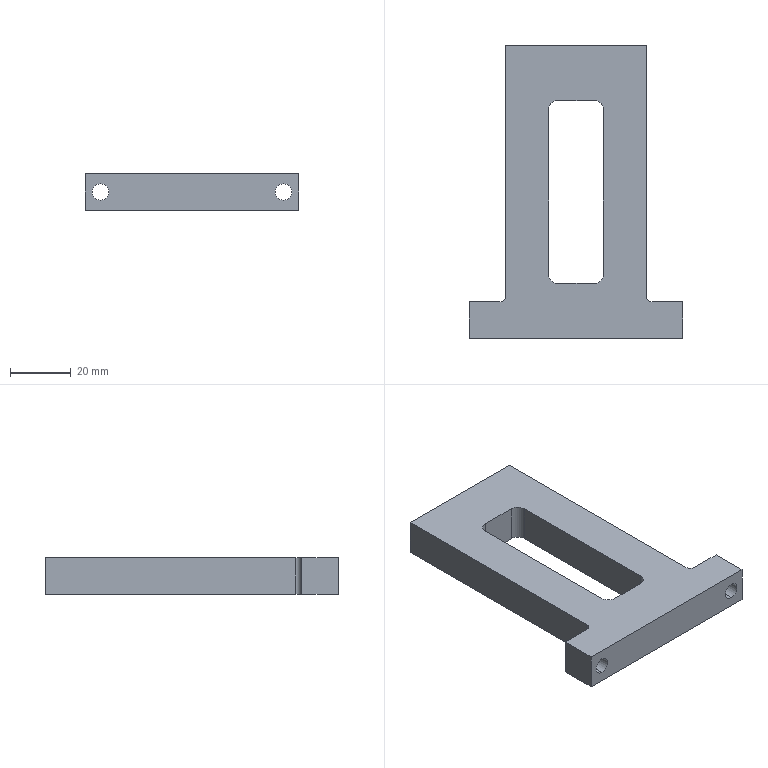Part | STEP file | 11-FG-E02011 | 1 solid | 36 faces | box 70 x 96 x 12 mm | volume 42748 mm3 | cylinder 16 | plane 14 | cone 6 | commonest cylinder face diameters 3.3 x6 5.4 x4 6 x4 4 x2
STEP:
#1=CARTESIAN_POINT('',(-17.,36.5,-1.65));
#2=VERTEX_POINT('',#1);
#3=CARTESIAN_POINT('',(-17.,36.5,1.65));
#4=VERTEX_POINT('',#3);
#5=CARTESIAN_POINT('',(-17.,36.5,0.));
#6=DIRECTION('',(0.,1.,0.));
#7=DIRECTION('',(0.,0.,1.));
#8=AXIS2_PLACEMENT_3D('',#5,#6,#7);
#9=CIRCLE('',#8,1.65);
#10=EDGE_CURVE('',#2,#4,#9,.T.);
#11=ORIENTED_EDGE('',*,*,#10,.F.);
#12=CARTESIAN_POINT('',(-17.,48.,-1.65));
#13=VERTEX_POINT('',#12);
#14=CARTESIAN_POINT('',(-17.,48.,-1.65));
#15=DIRECTION('',(0.,1.,0.));
#16=VECTOR('',#15,1000.);
#17=LINE('',#14,#16);
#18=EDGE_CURVE('',#2,#13,#17,.T.);
#19=ORIENTED_EDGE('',*,*,#18,.T.);
#20=CARTESIAN_POINT('',(-17.,48.,1.65));
#21=VERTEX_POINT('',#20);
#22=CARTESIAN_POINT('',(-17.,48.,0.));
#23=DIRECTION('',(0.,1.,0.));
#24=DIRECTION('',(0.,0.,1.));
#25=AXIS2_PLACEMENT_3D('',#22,#23,#24);
#26=CIRCLE('',#25,1.65);
#27=EDGE_CURVE('',#13,#21,#26,.T.);
#28=ORIENTED_EDGE('',*,*,#27,.T.);
#29=CARTESIAN_POINT('',(-17.,48.,1.65));
#30=DIRECTION('',(0.,1.,0.));
#31=VECTOR('',#30,1000.);
#32=LINE('',#29,#31);
#33=EDGE_CURVE('',#4,#21,#32,.T.);
#34=ORIENTED_EDGE('',*,*,#33,.F.);
#35=EDGE_LOOP('',(#11,#19,#28,#34));
#36=FACE_OUTER_BOUND('',#35,.T.);
#37=CARTESIAN_POINT('',(-17.,48.,0.));
#38=DIRECTION('',(0.,1.,0.));
#39=DIRECTION('',(0.,0.,1.));
#40=AXIS2_PLACEMENT_3D('',#37,#38,#39);
#41=CYLINDRICAL_SURFACE('',#40,1.65);
#42=ADVANCED_FACE('',(#36),#41,.F.);
#43=CARTESIAN_POINT('',(-17.,35.509,0.));
#44=VERTEX_POINT('',#43);
#45=CARTESIAN_POINT('',(-17.,36.5,1.65));
#46=DIRECTION('',(0.,0.515,0.8572));
#47=VECTOR('',#46,1000.);
#48=LINE('',#45,#47);
#49=EDGE_CURVE('',#44,#4,#48,.T.);
#50=ORIENTED_EDGE('',*,*,#49,.F.);
#51=CARTESIAN_POINT('',(-17.,36.5,-1.65));
#52=DIRECTION('',(0.,0.515,-0.8572));
#53=VECTOR('',#52,1000.);
#54=LINE('',#51,#53);
#55=EDGE_CURVE('',#44,#2,#54,.T.);
#56=ORIENTED_EDGE('',*,*,#55,.T.);
#57=ORIENTED_EDGE('',*,*,#10,.T.);
#58=EDGE_LOOP('',(#50,#56,#57));
#59=FACE_OUTER_BOUND('',#58,.T.);
#60=CARTESIAN_POINT('',(-17.,36.5,0.));
#61=DIRECTION('',(0.,1.,0.));
#62=DIRECTION('',(0.,0.,1.));
#63=AXIS2_PLACEMENT_3D('',#60,#61,#62);
#64=CONICAL_SURFACE('',#63,1.65,1.03);
#65=ADVANCED_FACE('',(#59),#64,.F.);
#66=CARTESIAN_POINT('',(0.,36.5,-1.65));
#67=VERTEX_POINT('',#66);
#68=CARTESIAN_POINT('',(0.,36.5,1.65));
#69=VERTEX_POINT('',#68);
#70=CARTESIAN_POINT('',(0.,36.5,0.));
#71=DIRECTION('',(0.,1.,0.));
#72=DIRECTION('',(0.,0.,1.));
#73=AXIS2_PLACEMENT_3D('',#70,#71,#72);
#74=CIRCLE('',#73,1.65);
#75=EDGE_CURVE('',#67,#69,#74,.T.);
#76=ORIENTED_EDGE('',*,*,#75,.F.);
#77=CARTESIAN_POINT('',(0.,48.,-1.65));
#78=VERTEX_POINT('',#77);
#79=CARTESIAN_POINT('',(0.,48.,-1.65));
#80=DIRECTION('',(0.,1.,0.));
#81=VECTOR('',#80,1000.);
#82=LINE('',#79,#81);
#83=EDGE_CURVE('',#67,#78,#82,.T.);
#84=ORIENTED_EDGE('',*,*,#83,.T.);
#85=CARTESIAN_POINT('',(0.,48.,1.65));
#86=VERTEX_POINT('',#85);
#87=CARTESIAN_POINT('',(0.,48.,0.));
#88=DIRECTION('',(0.,1.,0.));
#89=DIRECTION('',(0.,0.,1.));
#90=AXIS2_PLACEMENT_3D('',#87,#88,#89);
#91=CIRCLE('',#90,1.65);
#92=EDGE_CURVE('',#78,#86,#91,.T.);
#93=ORIENTED_EDGE('',*,*,#92,.T.);
#94=CARTESIAN_POINT('',(0.,48.,1.65));
#95=DIRECTION('',(0.,1.,0.));
#96=VECTOR('',#95,1000.);
#97=LINE('',#94,#96);
#98=EDGE_CURVE('',#69,#86,#97,.T.);
#99=ORIENTED_EDGE('',*,*,#98,.F.);
#100=EDGE_LOOP('',(#76,#84,#93,#99));
#101=FACE_OUTER_BOUND('',#100,.T.);
#102=CARTESIAN_POINT('',(0.,48.,0.));
#103=DIRECTION('',(0.,1.,0.));
#104=DIRECTION('',(0.,0.,1.));
#105=AXIS2_PLACEMENT_3D('',#102,#103,#104);
#106=CYLINDRICAL_SURFACE('',#105,1.65);
#107=ADVANCED_FACE('',(#101),#106,.F.);
#108=CARTESIAN_POINT('',(0.,35.509,0.));
#109=VERTEX_POINT('',#108);
#110=CARTESIAN_POINT('',(0.,36.5,1.65));
#111=DIRECTION('',(0.,0.515,0.8572));
#112=VECTOR('',#111,1000.);
#113=LINE('',#110,#112);
#114=EDGE_CURVE('',#109,#69,#113,.T.);
#115=ORIENTED_EDGE('',*,*,#114,.F.);
#116=CARTESIAN_POINT('',(0.,36.5,-1.65));
#117=DIRECTION('',(0.,0.515,-0.8572));
#118=VECTOR('',#117,1000.);
#119=LINE('',#116,#118);
#120=EDGE_CURVE('',#109,#67,#119,.T.);
#121=ORIENTED_EDGE('',*,*,#120,.T.);
#122=ORIENTED_EDGE('',*,*,#75,.T.);
#123=EDGE_LOOP('',(#115,#121,#122));
#124=FACE_OUTER_BOUND('',#123,.T.);
#125=CARTESIAN_POINT('',(0.,36.5,0.));
#126=DIRECTION('',(0.,1.,0.));
#127=DIRECTION('',(0.,0.,1.));
#128=AXIS2_PLACEMENT_3D('',#125,#126,#127);
#129=CONICAL_SURFACE('',#128,1.65,1.03);
#130=ADVANCED_FACE('',(#124),#129,.F.);
#131=CARTESIAN_POINT('',(17.,36.5,-1.65));
#132=VERTEX_POINT('',#131);
#133=CARTESIAN_POINT('',(17.,36.5,1.65));
#134=VERTEX_POINT('',#133);
#135=CARTESIAN_POINT('',(17.,36.5,0.));
#136=DIRECTION('',(0.,1.,0.));
#137=DIRECTION('',(0.,0.,1.));
#138=AXIS2_PLACEMENT_3D('',#135,#136,#137);
#139=CIRCLE('',#138,1.65);
#140=EDGE_CURVE('',#132,#134,#139,.T.);
#141=ORIENTED_EDGE('',*,*,#140,.F.);
#142=CARTESIAN_POINT('',(17.,48.,-1.65));
#143=VERTEX_POINT('',#142);
#144=CARTESIAN_POINT('',(17.,48.,-1.65));
#145=DIRECTION('',(0.,1.,0.));
#146=VECTOR('',#145,1000.);
#147=LINE('',#144,#146);
#148=EDGE_CURVE('',#132,#143,#147,.T.);
#149=ORIENTED_EDGE('',*,*,#148,.T.);
#150=CARTESIAN_POINT('',(17.,48.,1.65));
#151=VERTEX_POINT('',#150);
#152=CARTESIAN_POINT('',(17.,48.,0.));
#153=DIRECTION('',(0.,1.,0.));
#154=DIRECTION('',(0.,0.,1.));
#155=AXIS2_PLACEMENT_3D('',#152,#153,#154);
#156=CIRCLE('',#155,1.65);
#157=EDGE_CURVE('',#143,#151,#156,.T.);
#158=ORIENTED_EDGE('',*,*,#157,.T.);
#159=CARTESIAN_POINT('',(17.,48.,1.65));
#160=DIRECTION('',(0.,1.,0.));
#161=VECTOR('',#160,1000.);
#162=LINE('',#159,#161);
#163=EDGE_CURVE('',#134,#151,#162,.T.);
#164=ORIENTED_EDGE('',*,*,#163,.F.);
#165=EDGE_LOOP('',(#141,#149,#158,#164));
#166=FACE_OUTER_BOUND('',#165,.T.);
#167=CARTESIAN_POINT('',(17.,48.,0.));
#168=DIRECTION('',(0.,1.,0.));
#169=DIRECTION('',(0.,0.,1.));
#170=AXIS2_PLACEMENT_3D('',#167,#168,#169);
#171=CYLINDRICAL_SURFACE('',#170,1.65);
#172=ADVANCED_FACE('',(#166),#171,.F.);
#173=CARTESIAN_POINT('',(17.,35.509,0.));
#174=VERTEX_POINT('',#173);
#175=CARTESIAN_POINT('',(17.,36.5,1.65));
#176=DIRECTION('',(0.,0.515,0.8572));
#177=VECTOR('',#176,1000.);
#178=LINE('',#175,#177);
#179=EDGE_CURVE('',#174,#134,#178,.T.);
#180=ORIENTED_EDGE('',*,*,#179,.F.);
#181=CARTESIAN_POINT('',(17.,36.5,-1.65));
#182=DIRECTION('',(0.,0.515,-0.8572));
#183=VECTOR('',#182,1000.);
#184=LINE('',#181,#183);
#185=EDGE_CURVE('',#174,#132,#184,.T.);
#186=ORIENTED_EDGE('',*,*,#185,.T.);
#187=ORIENTED_EDGE('',*,*,#140,.T.);
#188=EDGE_LOOP('',(#180,#186,#187));
#189=FACE_OUTER_BOUND('',#188,.T.);
#190=CARTESIAN_POINT('',(17.,36.5,0.));
#191=DIRECTION('',(0.,1.,0.));
#192=DIRECTION('',(0.,0.,1.));
#193=AXIS2_PLACEMENT_3D('',#190,#191,#192);
#194=CONICAL_SURFACE('',#193,1.65,1.03);
#195=ADVANCED_FACE('',(#189),#194,.F.);
#196=CARTESIAN_POINT('',(30.,-48.,-2.7));
#197=VERTEX_POINT('',#196);
#198=CARTESIAN_POINT('',(30.,-48.,2.7));
#199=VERTEX_POINT('',#198);
#200=CARTESIAN_POINT('',(30.,-48.,0.));
#201=DIRECTION('',(0.,1.,0.));
#202=DIRECTION('',(0.,0.,1.));
#203=AXIS2_PLACEMENT_3D('',#200,#201,#202);
#204=CIRCLE('',#203,2.7);
#205=EDGE_CURVE('',#197,#199,#204,.T.);
#206=ORIENTED_EDGE('',*,*,#205,.F.);
#207=CARTESIAN_POINT('',(30.,-36.,-2.7));
#208=VERTEX_POINT('',#207);
#209=CARTESIAN_POINT('',(30.,-36.,-2.7));
#210=DIRECTION('',(0.,1.,0.));
#211=VECTOR('',#210,1000.);
#212=LINE('',#209,#211);
#213=EDGE_CURVE('',#197,#208,#212,.T.);
#214=ORIENTED_EDGE('',*,*,#213,.T.);
#215=CARTESIAN_POINT('',(30.,-36.,2.7));
#216=VERTEX_POINT('',#215);
#217=CARTESIAN_POINT('',(30.,-36.,0.));
#218=DIRECTION('',(0.,1.,0.));
#219=DIRECTION('',(0.,0.,1.));
#220=AXIS2_PLACEMENT_3D('',#217,#218,#219);
#221=CIRCLE('',#220,2.7);
#222=EDGE_CURVE('',#208,#216,#221,.T.);
#223=ORIENTED_EDGE('',*,*,#222,.T.);
#224=CARTESIAN_POINT('',(30.,-36.,2.7));
#225=DIRECTION('',(0.,1.,0.));
#226=VECTOR('',#225,1000.);
#227=LINE('',#224,#226);
#228=EDGE_CURVE('',#199,#216,#227,.T.);
#229=ORIENTED_EDGE('',*,*,#228,.F.);
#230=EDGE_LOOP('',(#206,#214,#223,#229));
#231=FACE_OUTER_BOUND('',#230,.T.);
#232=CARTESIAN_POINT('',(30.,-36.,0.));
#233=DIRECTION('',(0.,1.,0.));
#234=DIRECTION('',(0.,0.,1.));
#235=AXIS2_PLACEMENT_3D('',#232,#233,#234);
#236=CYLINDRICAL_SURFACE('',#235,2.7);
#237=ADVANCED_FACE('',(#231),#236,.F.);
#238=CARTESIAN_POINT('',(-30.,-48.,-2.7));
#239=VERTEX_POINT('',#238);
#240=CARTESIAN_POINT('',(-30.,-48.,2.7));
#241=VERTEX_POINT('',#240);
#242=CARTESIAN_POINT('',(-30.,-48.,0.));
#243=DIRECTION('',(0.,1.,0.));
#244=DIRECTION('',(0.,0.,1.));
#245=AXIS2_PLACEMENT_3D('',#242,#243,#244);
#246=CIRCLE('',#245,2.7);
#247=EDGE_CURVE('',#239,#241,#246,.T.);
#248=ORIENTED_EDGE('',*,*,#247,.F.);
#249=CARTESIAN_POINT('',(-30.,-36.,-2.7));
#250=VERTEX_POINT('',#249);
#251=CARTESIAN_POINT('',(-30.,-36.,-2.7));
#252=DIRECTION('',(0.,1.,0.));
#253=VECTOR('',#252,1000.);
#254=LINE('',#251,#253);
#255=EDGE_CURVE('',#239,#250,#254,.T.);
#256=ORIENTED_EDGE('',*,*,#255,.T.);
#257=CARTESIAN_POINT('',(-30.,-36.,2.7));
#258=VERTEX_POINT('',#257);
#259=CARTESIAN_POINT('',(-30.,-36.,0.));
#260=DIRECTION('',(0.,1.,0.));
#261=DIRECTION('',(0.,0.,1.));
#262=AXIS2_PLACEMENT_3D('',#259,#260,#261);
#263=CIRCLE('',#262,2.7);
#264=EDGE_CURVE('',#250,#258,#263,.T.);
#265=ORIENTED_EDGE('',*,*,#264,.T.);
#266=CARTESIAN_POINT('',(-30.,-36.,2.7));
#267=DIRECTION('',(0.,1.,0.));
#268=VECTOR('',#267,1000.);
#269=LINE('',#266,#268);
#270=EDGE_CURVE('',#241,#258,#269,.T.);
#271=ORIENTED_EDGE('',*,*,#270,.F.);
#272=EDGE_LOOP('',(#248,#256,#265,#271));
#273=FACE_OUTER_BOUND('',#272,.T.);
#274=CARTESIAN_POINT('',(-30.,-36.,0.));
#275=DIRECTION('',(0.,1.,0.));
#276=DIRECTION('',(0.,0.,1.));
#277=AXIS2_PLACEMENT_3D('',#274,#275,#276);
#278=CYLINDRICAL_SURFACE('',#277,2.7);
#279=ADVANCED_FACE('',(#273),#278,.F.);
#280=CARTESIAN_POINT('',(35.,-48.,-6.));
#281=VERTEX_POINT('',#280);
#282=CARTESIAN_POINT('',(35.,-36.,-6.));
#283=VERTEX_POINT('',#282);
#284=CARTESIAN_POINT('',(35.,-48.,-6.));
#285=DIRECTION('',(0.,1.,0.));
#286=VECTOR('',#285,1000.);
#287=LINE('',#284,#286);
#288=EDGE_CURVE('',#281,#283,#287,.T.);
#289=ORIENTED_EDGE('',*,*,#288,.T.);
#290=CARTESIAN_POINT('',(35.,-36.,6.));
#291=VERTEX_POINT('',#290);
#292=CARTESIAN_POINT('',(35.,-36.,-6.));
#293=DIRECTION('',(0.,0.,1.));
#294=VECTOR('',#293,1000.);
#295=LINE('',#292,#294);
#296=EDGE_CURVE('',#283,#291,#295,.T.);
#297=ORIENTED_EDGE('',*,*,#296,.T.);
#298=CARTESIAN_POINT('',(35.,-48.,6.));
#299=VERTEX_POINT('',#298);
#300=CARTESIAN_POINT('',(35.,-48.,6.));
#301=DIRECTION('',(0.,1.,0.));
#302=VECTOR('',#301,1000.);
#303=LINE('',#300,#302);
#304=EDGE_CURVE('',#299,#291,#303,.T.);
#305=ORIENTED_EDGE('',*,*,#304,.F.);
#306=CARTESIAN_POINT('',(35.,-48.,6.));
#307=DIRECTION('',(0.,0.,-1.));
#308=VECTOR('',#307,1000.);
#309=LINE('',#306,#308);
#310=EDGE_CURVE('',#299,#281,#309,.T.);
#311=ORIENTED_EDGE('',*,*,#310,.T.);
#312=EDGE_LOOP('',(#289,#297,#305,#311));
#313=FACE_OUTER_BOUND('',#312,.T.);
#314=CARTESIAN_POINT('',(35.,-48.,6.));
#315=DIRECTION('',(-1.,0.,0.));
#316=DIRECTION('',(0.,0.,1.));
#317=AXIS2_PLACEMENT_3D('',#314,#315,#316);
#318=PLANE('',#317);
#319=ADVANCED_FACE('',(#313),#318,.F.);
#320=CARTESIAN_POINT('',(-17.,48.,0.));
#321=DIRECTION('',(0.,1.,0.));
#322=DIRECTION('',(0.,0.,1.));
#323=AXIS2_PLACEMENT_3D('',#320,#321,#322);
#324=CIRCLE('',#323,1.65);
#325=EDGE_CURVE('',#21,#13,#324,.T.);
#326=ORIENTED_EDGE('',*,*,#325,.F.);
#327=ORIENTED_EDGE('',*,*,#27,.F.);
#328=EDGE_LOOP('',(#326,#327));
#329=FACE_BOUND('',#328,.T.);
#330=CARTESIAN_POINT('',(0.,48.,0.));
#331=DIRECTION('',(0.,1.,0.));
#332=DIRECTION('',(0.,0.,1.));
#333=AXIS2_PLACEMENT_3D('',#330,#331,#332);
#334=CIRCLE('',#333,1.65);
#335=EDGE_CURVE('',#86,#78,#334,.T.);
#336=ORIENTED_EDGE('',*,*,#335,.F.);
#337=ORIENTED_EDGE('',*,*,#92,.F.);
#338=EDGE_LOOP('',(#336,#337));
#339=FACE_BOUND('',#338,.T.);
#340=CARTESIAN_POINT('',(17.,48.,0.));
#341=DIRECTION('',(0.,1.,0.));
#342=DIRECTION('',(0.,0.,1.));
#343=AXIS2_PLACEMENT_3D('',#340,#341,#342);
#344=CIRCLE('',#343,1.65);
#345=EDGE_CURVE('',#151,#143,#344,.T.);
#346=ORIENTED_EDGE('',*,*,#345,.F.);
#347=ORIENTED_EDGE('',*,*,#157,.F.);
#348=EDGE_LOOP('',(#346,#347));
#349=FACE_BOUND('',#348,.T.);
#350=CARTESIAN_POINT('',(23.,48.,-6.));
#351=VERTEX_POINT('',#350);
#352=CARTESIAN_POINT('',(-23.,48.,-6.));
#353=VERTEX_POINT('',#352);
#354=CARTESIAN_POINT('',(-35.,48.,-6.));
#355=DIRECTION('',(-1.,0.,0.));
#356=VECTOR('',#355,1000.);
#357=LINE('',#354,#356);
#358=EDGE_CURVE('',#351,#353,#357,.T.);
#359=ORIENTED_EDGE('',*,*,#358,.T.);
#360=CARTESIAN_POINT('',(-23.,48.,6.));
#361=VERTEX_POINT('',#360);
#362=CARTESIAN_POINT('',(-23.,48.,-6.));
#363=DIRECTION('',(0.,0.,1.));
#364=VECTOR('',#363,1000.);
#365=LINE('',#362,#364);
#366=EDGE_CURVE('',#353,#361,#365,.T.);
#367=ORIENTED_EDGE('',*,*,#366,.T.);
#368=CARTESIAN_POINT('',(23.,48.,6.));
#369=VERTEX_POINT('',#368);
#370=CARTESIAN_POINT('',(-35.,48.,6.));
#371=DIRECTION('',(-1.,0.,0.));
#372=VECTOR('',#371,1000.);
#373=LINE('',#370,#372);
#374=EDGE_CURVE('',#369,#361,#373,.T.);
#375=ORIENTED_EDGE('',*,*,#374,.F.);
#376=CARTESIAN_POINT('',(23.,48.,-6.));
#377=DIRECTION('',(0.,0.,1.));
#378=VECTOR('',#377,1000.);
#379=LINE('',#376,#378);
#380=EDGE_CURVE('',#351,#369,#379,.T.);
#381=ORIENTED_EDGE('',*,*,#380,.F.);
#382=EDGE_LOOP('',(#359,#367,#375,#381));
#383=FACE_OUTER_BOUND('',#382,.T.);
#384=CARTESIAN_POINT('',(-35.,48.,6.));
#385=DIRECTION('',(0.,-1.,0.));
#386=DIRECTION('',(0.,0.,-1.));
#387=AXIS2_PLACEMENT_3D('',#384,#385,#386);
#388=PLANE('',#387);
#389=ADVANCED_FACE('',(#329,#339,#349,#383),#388,.F.);
#390=CARTESIAN_POINT('',(-35.,-36.,6.));
#391=VERTEX_POINT('',#390);
#392=CARTESIAN_POINT('',(-35.,-48.,6.));
#393=VERTEX_POINT('',#392);
#394=CARTESIAN_POINT('',(-35.,-48.,6.));
#395=DIRECTION('',(0.,-1.,0.));
#396=VECTOR('',#395,1000.);
#397=LINE('',#394,#396);
#398=EDGE_CURVE('',#391,#393,#397,.T.);
#399=ORIENTED_EDGE('',*,*,#398,.F.);
#400=CARTESIAN_POINT('',(-35.,-36.,-6.));
#401=VERTEX_POINT('',#400);
#402=CARTESIAN_POINT('',(-35.,-36.,-6.));
#403=DIRECTION('',(0.,0.,1.));
#404=VECTOR('',#403,1000.);
#405=LINE('',#402,#404);
#406=EDGE_CURVE('',#401,#391,#405,.T.);
#407=ORIENTED_EDGE('',*,*,#406,.F.);
#408=CARTESIAN_POINT('',(-35.,-48.,-6.));
#409=VERTEX_POINT('',#408);
#410=CARTESIAN_POINT('',(-35.,-48.,-6.));
#411=DIRECTION('',(0.,-1.,0.));
#412=VECTOR('',#411,1000.);
#413=LINE('',#410,#412);
#414=EDGE_CURVE('',#401,#409,#413,.T.);
#415=ORIENTED_EDGE('',*,*,#414,.T.);
#416=CARTESIAN_POINT('',(-35.,-48.,6.));
#417=DIRECTION('',(0.,0.,-1.));
#418=VECTOR('',#417,1000.);
#419=LINE('',#416,#418);
#420=EDGE_CURVE('',#393,#409,#419,.T.);
#421=ORIENTED_EDGE('',*,*,#420,.F.);
#422=EDGE_LOOP('',(#399,#407,#415,#421));
#423=FACE_OUTER_BOUND('',#422,.T.);
#424=CARTESIAN_POINT('',(-35.,-48.,6.));
#425=DIRECTION('',(1.,0.,0.));
#426=DIRECTION('',(0.,0.,-1.));
#427=AXIS2_PLACEMENT_3D('',#424,#425,#426);
#428=PLANE('',#427);
#429=ADVANCED_FACE('',(#423),#428,.F.);
#430=CARTESIAN_POINT('',(30.,-48.,0.));
#431=DIRECTION('',(0.,1.,0.));
#432=DIRECTION('',(0.,0.,1.));
#433=AXIS2_PLACEMENT_3D('',#430,#431,#432);
#434=CIRCLE('',#433,2.7);
#435=EDGE_CURVE('',#199,#197,#434,.T.);
#436=ORIENTED_EDGE('',*,*,#435,.T.);
#437=ORIENTED_EDGE('',*,*,#205,.T.);
#438=EDGE_LOOP('',(#436,#437));
#439=FACE_BOUND('',#438,.T.);
#440=CARTESIAN_POINT('',(-30.,-48.,0.));
#441=DIRECTION('',(0.,1.,0.));
#442=DIRECTION('',(0.,0.,1.));
#443=AXIS2_PLACEMENT_3D('',#440,#441,#442);
#444=CIRCLE('',#443,2.7);
#445=EDGE_CURVE('',#241,#239,#444,.T.);
#446=ORIENTED_EDGE('',*,*,#445,.T.);
#447=ORIENTED_EDGE('',*,*,#247,.T.);
#448=EDGE_LOOP('',(#446,#447));
#449=FACE_BOUND('',#448,.T.);
#450=CARTESIAN_POINT('',(-35.,-48.,-6.));
#451=DIRECTION('',(1.,0.,0.));
#452=VECTOR('',#451,1000.);
#453=LINE('',#450,#452);
#454=EDGE_CURVE('',#409,#281,#453,.T.);
#455=ORIENTED_EDGE('',*,*,#454,.T.);
#456=ORIENTED_EDGE('',*,*,#310,.F.);
#457=CARTESIAN_POINT('',(-35.,-48.,6.));
#458=DIRECTION('',(1.,0.,0.));
#459=VECTOR('',#458,1000.);
#460=LINE('',#457,#459);
#461=EDGE_CURVE('',#393,#299,#460,.T.);
#462=ORIENTED_EDGE('',*,*,#461,.F.);
#463=ORIENTED_EDGE('',*,*,#420,.T.);
#464=EDGE_LOOP('',(#455,#456,#462,#463));
#465=FACE_OUTER_BOUND('',#464,.T.);
#466=CARTESIAN_POINT('',(-35.,-48.,6.));
#467=DIRECTION('',(0.,1.,0.));
#468=DIRECTION('',(0.,0.,1.));
#469=AXIS2_PLACEMENT_3D('',#466,#467,#468);
#470=PLANE('',#469);
#471=ADVANCED_FACE('',(#439,#449,#465),#470,.F.);
#472=CARTESIAN_POINT('',(9.,-27.,6.));
#473=VERTEX_POINT('',#472);
#474=CARTESIAN_POINT('',(9.,27.,6.));
#475=VERTEX_POINT('',#474);
#476=CARTESIAN_POINT('',(9.,-27.,6.));
#477=DIRECTION('',(0.,1.,0.));
#478=VECTOR('',#477,1000.);
#479=LINE('',#476,#478);
#480=EDGE_CURVE('',#473,#475,#479,.T.);
#481=ORIENTED_EDGE('',*,*,#480,.F.);
#482=CARTESIAN_POINT('',(6.,-30.,6.));
#483=VERTEX_POINT('',#482);
#484=CARTESIAN_POINT('',(6.,-27.,6.));
#485=DIRECTION('',(0.,0.,1.));
#486=DIRECTION('',(1.,0.,0.));
#487=AXIS2_PLACEMENT_3D('',#484,#485,#486);
#488=CIRCLE('',#487,3.);
#489=EDGE_CURVE('',#483,#473,#488,.T.);
#490=ORIENTED_EDGE('',*,*,#489,.F.);
#491=CARTESIAN_POINT('',(-6.,-30.,6.));
#492=VERTEX_POINT('',#491);
#493=CARTESIAN_POINT('',(-6.,-30.,6.));
#494=DIRECTION('',(1.,0.,0.));
#495=VECTOR('',#494,1000.);
#496=LINE('',#493,#495);
#497=EDGE_CURVE('',#492,#483,#496,.T.);
#498=ORIENTED_EDGE('',*,*,#497,.F.);
#499=CARTESIAN_POINT('',(-9.,-27.,6.));
#500=VERTEX_POINT('',#499);
#501=CARTESIAN_POINT('',(-6.,-27.,6.));
#502=DIRECTION('',(0.,0.,1.));
#503=DIRECTION('',(-1.,0.,0.));
#504=AXIS2_PLACEMENT_3D('',#501,#502,#503);
#505=CIRCLE('',#504,3.);
#506=EDGE_CURVE('',#500,#492,#505,.T.);
#507=ORIENTED_EDGE('',*,*,#506,.F.);
#508=CARTESIAN_POINT('',(-9.,27.,6.));
#509=VERTEX_POINT('',#508);
#510=CARTESIAN_POINT('',(-9.,-27.,6.));
#511=DIRECTION('',(0.,-1.,0.));
#512=VECTOR('',#511,1000.);
#513=LINE('',#510,#512);
#514=EDGE_CURVE('',#509,#500,#513,.T.);
#515=ORIENTED_EDGE('',*,*,#514,.F.);
#516=CARTESIAN_POINT('',(-6.,30.,6.));
#517=VERTEX_POINT('',#516);
#518=CARTESIAN_POINT('',(-6.,27.,6.));
#519=DIRECTION('',(0.,0.,1.));
#520=DIRECTION('',(-1.,0.,0.));
#521=AXIS2_PLACEMENT_3D('',#518,#519,#520);
#522=CIRCLE('',#521,3.);
#523=EDGE_CURVE('',#517,#509,#522,.T.);
#524=ORIENTED_EDGE('',*,*,#523,.F.);
#525=CARTESIAN_POINT('',(6.,30.,6.));
#526=VERTEX_POINT('',#525);
#527=CARTESIAN_POINT('',(-6.,30.,6.));
#528=DIRECTION('',(-1.,0.,0.));
#529=VECTOR('',#528,1000.);
#530=LINE('',#527,#529);
#531=EDGE_CURVE('',#526,#517,#530,.T.);
#532=ORIENTED_EDGE('',*,*,#531,.F.);
#533=CARTESIAN_POINT('',(6.,27.,6.));
#534=DIRECTION('',(0.,0.,1.));
#535=DIRECTION('',(-1.,0.,0.));
#536=AXIS2_PLACEMENT_3D('',#533,#534,#535);
#537=CIRCLE('',#536,3.);
#538=EDGE_CURVE('',#475,#526,#537,.T.);
#539=ORIENTED_EDGE('',*,*,#538,.F.);
#540=EDGE_LOOP('',(#481,#490,#498,#507,#515,#524,#532,#539));
#541=FACE_BOUND('',#540,.T.);
#542=ORIENTED_EDGE('',*,*,#374,.T.);
#543=CARTESIAN_POINT('',(-23.,-34.,6.));
#544=VERTEX_POINT('',#543);
#545=CARTESIAN_POINT('',(-23.,48.,6.));
#546=DIRECTION('',(0.,1.,0.));
#547=VECTOR('',#546,1000.);
#548=LINE('',#545,#547);
#549=EDGE_CURVE('',#544,#361,#548,.T.);
#550=ORIENTED_EDGE('',*,*,#549,.F.);
#551=CARTESIAN_POINT('',(-25.,-36.,6.));
#552=VERTEX_POINT('',#551);
#553=CARTESIAN_POINT('',(-25.,-34.,6.));
#554=DIRECTION('',(0.,0.,1.));
#555=DIRECTION('',(-1.,0.,0.));
#556=AXIS2_PLACEMENT_3D('',#553,#554,#555);
#557=CIRCLE('',#556,2.);
#558=EDGE_CURVE('',#552,#544,#557,.T.);
#559=ORIENTED_EDGE('',*,*,#558,.F.);
#560=CARTESIAN_POINT('',(-35.,-36.,6.));
#561=DIRECTION('',(1.,0.,0.));
#562=VECTOR('',#561,1000.);
#563=LINE('',#560,#562);
#564=EDGE_CURVE('',#391,#552,#563,.T.);
#565=ORIENTED_EDGE('',*,*,#564,.F.);
#566=ORIENTED_EDGE('',*,*,#398,.T.);
#567=ORIENTED_EDGE('',*,*,#461,.T.);
#568=ORIENTED_EDGE('',*,*,#304,.T.);
#569=CARTESIAN_POINT('',(25.,-36.,6.));
#570=VERTEX_POINT('',#569);
#571=CARTESIAN_POINT('',(35.,-36.,6.));
#572=DIRECTION('',(1.,0.,0.));
#573=VECTOR('',#572,1000.);
#574=LINE('',#571,#573);
#575=EDGE_CURVE('',#570,#291,#574,.T.);
#576=ORIENTED_EDGE('',*,*,#575,.F.);
#577=CARTESIAN_POINT('',(23.,-34.,6.));
#578=VERTEX_POINT('',#577);
#579=CARTESIAN_POINT('',(25.,-34.,6.));
#580=DIRECTION('',(0.,0.,1.));
#581=DIRECTION('',(-1.,0.,0.));
#582=AXIS2_PLACEMENT_3D('',#579,#580,#581);
#583=CIRCLE('',#582,2.);
#584=EDGE_CURVE('',#578,#570,#583,.T.);
#585=ORIENTED_EDGE('',*,*,#584,.F.);
#586=CARTESIAN_POINT('',(23.,48.,6.));
#587=DIRECTION('',(0.,-1.,0.));
#588=VECTOR('',#587,1000.);
#589=LINE('',#586,#588);
#590=EDGE_CURVE('',#369,#578,#589,.T.);
#591=ORIENTED_EDGE('',*,*,#590,.F.);
#592=EDGE_LOOP('',(#542,#550,#559,#565,#566,#567,#568,#576,#585,#591));
#593=FACE_OUTER_BOUND('',#592,.T.);
#594=CARTESIAN_POINT('',(0.,0.,6.));
#595=DIRECTION('',(0.,0.,-1.));
#596=DIRECTION('',(-1.,0.,0.));
#597=AXIS2_PLACEMENT_3D('',#594,#595,#596);
#598=PLANE('',#597);
#599=ADVANCED_FACE('',(#541,#593),#598,.F.);
#600=CARTESIAN_POINT('',(6.,-30.,-6.));
#601=VERTEX_POINT('',#600);
#602=CARTESIAN_POINT('',(9.,-27.,-6.));
#603=VERTEX_POINT('',#602);
#604=CARTESIAN_POINT('',(6.,-27.,-6.));
#605=DIRECTION('',(0.,0.,1.));
#606=DIRECTION('',(1.,0.,0.));
#607=AXIS2_PLACEMENT_3D('',#604,#605,#606);
#608=CIRCLE('',#607,3.);
#609=EDGE_CURVE('',#601,#603,#608,.T.);
#610=ORIENTED_EDGE('',*,*,#609,.T.);
#611=CARTESIAN_POINT('',(9.,27.,-6.));
#612=VERTEX_POINT('',#611);
#613=CARTESIAN_POINT('',(9.,-27.,-6.));
#614=DIRECTION('',(0.,1.,0.));
#615=VECTOR('',#614,1000.);
#616=LINE('',#613,#615);
#617=EDGE_CURVE('',#603,#612,#616,.T.);
#618=ORIENTED_EDGE('',*,*,#617,.T.);
#619=CARTESIAN_POINT('',(6.,30.,-6.));
#620=VERTEX_POINT('',#619);
#621=CARTESIAN_POINT('',(6.,27.,-6.));
#622=DIRECTION('',(0.,0.,1.));
#623=DIRECTION('',(-1.,0.,0.));
#624=AXIS2_PLACEMENT_3D('',#621,#622,#623);
#625=CIRCLE('',#624,3.);
#626=EDGE_CURVE('',#612,#620,#625,.T.);
#627=ORIENTED_EDGE('',*,*,#626,.T.);
#628=CARTESIAN_POINT('',(-6.,30.,-6.));
#629=VERTEX_POINT('',#628);
#630=CARTESIAN_POINT('',(-6.,30.,-6.));
#631=DIRECTION('',(-1.,0.,0.));
#632=VECTOR('',#631,1000.);
#633=LINE('',#630,#632);
#634=EDGE_CURVE('',#620,#629,#633,.T.);
#635=ORIENTED_EDGE('',*,*,#634,.T.);
#636=CARTESIAN_POINT('',(-9.,27.,-6.));
#637=VERTEX_POINT('',#636);
#638=CARTESIAN_POINT('',(-6.,27.,-6.));
#639=DIRECTION('',(0.,0.,1.));
#640=DIRECTION('',(-1.,0.,0.));
#641=AXIS2_PLACEMENT_3D('',#638,#639,#640);
#642=CIRCLE('',#641,3.);
#643=EDGE_CURVE('',#629,#637,#642,.T.);
#644=ORIENTED_EDGE('',*,*,#643,.T.);
#645=CARTESIAN_POINT('',(-9.,-27.,-6.));
#646=VERTEX_POINT('',#645);
#647=CARTESIAN_POINT('',(-9.,-27.,-6.));
#648=DIRECTION('',(0.,-1.,0.));
#649=VECTOR('',#648,1000.);
#650=LINE('',#647,#649);
#651=EDGE_CURVE('',#637,#646,#650,.T.);
#652=ORIENTED_EDGE('',*,*,#651,.T.);
#653=CARTESIAN_POINT('',(-6.,-30.,-6.));
#654=VERTEX_POINT('',#653);
#655=CARTESIAN_POINT('',(-6.,-27.,-6.));
#656=DIRECTION('',(0.,0.,1.));
#657=DIRECTION('',(-1.,0.,0.));
#658=AXIS2_PLACEMENT_3D('',#655,#656,#657);
#659=CIRCLE('',#658,3.);
#660=EDGE_CURVE('',#646,#654,#659,.T.);
#661=ORIENTED_EDGE('',*,*,#660,.T.);
#662=CARTESIAN_POINT('',(-6.,-30.,-6.));
#663=DIRECTION('',(1.,0.,0.));
#664=VECTOR('',#663,1000.);
#665=LINE('',#662,#664);
#666=EDGE_CURVE('',#654,#601,#665,.T.);
#667=ORIENTED_EDGE('',*,*,#666,.T.);
#668=EDGE_LOOP('',(#610,#618,#627,#635,#644,#652,#661,#667));
#669=FACE_BOUND('',#668,.T.);
#670=CARTESIAN_POINT('',(-23.,-34.,-6.));
#671=VERTEX_POINT('',#670);
#672=CARTESIAN_POINT('',(-23.,48.,-6.));
#673=DIRECTION('',(0.,1.,0.));
#674=VECTOR('',#673,1000.);
#675=LINE('',#672,#674);
#676=EDGE_CURVE('',#671,#353,#675,.T.);
#677=ORIENTED_EDGE('',*,*,#676,.T.);
#678=ORIENTED_EDGE('',*,*,#358,.F.);
#679=CARTESIAN_POINT('',(23.,-34.,-6.));
#680=VERTEX_POINT('',#679);
#681=CARTESIAN_POINT('',(23.,48.,-6.));
#682=DIRECTION('',(0.,-1.,0.));
#683=VECTOR('',#682,1000.);
#684=LINE('',#681,#683);
#685=EDGE_CURVE('',#351,#680,#684,.T.);
#686=ORIENTED_EDGE('',*,*,#685,.T.);
#687=CARTESIAN_POINT('',(25.,-36.,-6.));
#688=VERTEX_POINT('',#687);
#689=CARTESIAN_POINT('',(25.,-34.,-6.));
#690=DIRECTION('',(0.,0.,1.));
#691=DIRECTION('',(-1.,0.,0.));
#692=AXIS2_PLACEMENT_3D('',#689,#690,#691);
#693=CIRCLE('',#692,2.);
#694=EDGE_CURVE('',#680,#688,#693,.T.);
#695=ORIENTED_EDGE('',*,*,#694,.T.);
#696=CARTESIAN_POINT('',(35.,-36.,-6.));
#697=DIRECTION('',(1.,0.,0.));
#698=VECTOR('',#697,1000.);
#699=LINE('',#696,#698);
#700=EDGE_CURVE('',#688,#283,#699,.T.);
#701=ORIENTED_EDGE('',*,*,#700,.T.);
#702=ORIENTED_EDGE('',*,*,#288,.F.);
#703=ORIENTED_EDGE('',*,*,#454,.F.);
#704=ORIENTED_EDGE('',*,*,#414,.F.);
#705=CARTESIAN_POINT('',(-25.,-36.,-6.));
#706=VERTEX_POINT('',#705);
#707=CARTESIAN_POINT('',(-35.,-36.,-6.));
#708=DIRECTION('',(1.,0.,0.));
#709=VECTOR('',#708,1000.);
#710=LINE('',#707,#709);
#711=EDGE_CURVE('',#401,#706,#710,.T.);
#712=ORIENTED_EDGE('',*,*,#711,.T.);
#713=CARTESIAN_POINT('',(-25.,-34.,-6.));
#714=DIRECTION('',(0.,0.,1.));
#715=DIRECTION('',(-1.,0.,0.));
#716=AXIS2_PLACEMENT_3D('',#713,#714,#715);
#717=CIRCLE('',#716,2.);
#718=EDGE_CURVE('',#706,#671,#717,.T.);
#719=ORIENTED_EDGE('',*,*,#718,.T.);
#720=EDGE_LOOP('',(#677,#678,#686,#695,#701,#702,#703,#704,#712,#719));
#721=FACE_OUTER_BOUND('',#720,.T.);
#722=CARTESIAN_POINT('',(0.,0.,-6.));
#723=DIRECTION('',(0.,0.,-1.));
#724=DIRECTION('',(-1.,0.,0.));
#725=AXIS2_PLACEMENT_3D('',#722,#723,#724);
#726=PLANE('',#725);
#727=ADVANCED_FACE('',(#669,#721),#726,.T.);
#728=CARTESIAN_POINT('',(30.,-36.,0.));
#729=DIRECTION('',(0.,1.,0.));
#730=DIRECTION('',(0.,0.,1.));
#731=AXIS2_PLACEMENT_3D('',#728,#729,#730);
#732=CIRCLE('',#731,2.7);
#733=EDGE_CURVE('',#216,#208,#732,.T.);
#734=ORIENTED_EDGE('',*,*,#733,.F.);
#735=ORIENTED_EDGE('',*,*,#222,.F.);
#736=EDGE_LOOP('',(#734,#735));
#737=FACE_BOUND('',#736,.T.);
#738=ORIENTED_EDGE('',*,*,#575,.T.);
#739=ORIENTED_EDGE('',*,*,#296,.F.);
#740=ORIENTED_EDGE('',*,*,#700,.F.);
#741=CARTESIAN_POINT('',(25.,-36.,-6.));
#742=DIRECTION('',(0.,0.,1.));
#743=VECTOR('',#742,1000.);
#744=LINE('',#741,#743);
#745=EDGE_CURVE('',#688,#570,#744,.T.);
#746=ORIENTED_EDGE('',*,*,#745,.T.);
#747=EDGE_LOOP('',(#738,#739,#740,#746));
#748=FACE_OUTER_BOUND('',#747,.T.);
#749=CARTESIAN_POINT('',(35.,-36.,-6.));
#750=DIRECTION('',(0.,-1.,0.));
#751=DIRECTION('',(1.,0.,0.));
#752=AXIS2_PLACEMENT_3D('',#749,#750,#751);
#753=PLANE('',#752);
#754=ADVANCED_FACE('',(#737,#748),#753,.F.);
#755=ORIENTED_EDGE('',*,*,#584,.T.);
#756=ORIENTED_EDGE('',*,*,#745,.F.);
#757=ORIENTED_EDGE('',*,*,#694,.F.);
#758=CARTESIAN_POINT('',(23.,-34.,-6.));
#759=DIRECTION('',(0.,0.,1.));
#760=VECTOR('',#759,1000.);
#761=LINE('',#758,#760);
#762=EDGE_CURVE('',#680,#578,#761,.T.);
#763=ORIENTED_EDGE('',*,*,#762,.T.);
#764=EDGE_LOOP('',(#755,#756,#757,#763));
#765=FACE_OUTER_BOUND('',#764,.T.);
#766=CARTESIAN_POINT('',(25.,-34.,-6.));
#767=DIRECTION('',(0.,0.,1.));
#768=DIRECTION('',(1.,0.,0.));
#769=AXIS2_PLACEMENT_3D('',#766,#767,#768);
#770=CYLINDRICAL_SURFACE('',#769,2.);
#771=ADVANCED_FACE('',(#765),#770,.F.);
#772=ORIENTED_EDGE('',*,*,#590,.T.);
#773=ORIENTED_EDGE('',*,*,#762,.F.);
#774=ORIENTED_EDGE('',*,*,#685,.F.);
#775=ORIENTED_EDGE('',*,*,#380,.T.);
#776=EDGE_LOOP('',(#772,#773,#774,#775));
#777=FACE_OUTER_BOUND('',#776,.T.);
#778=CARTESIAN_POINT('',(23.,48.,-6.));
#779=DIRECTION('',(-1.,0.,0.));
#780=DIRECTION('',(0.,-1.,0.));
#781=AXIS2_PLACEMENT_3D('',#778,#779,#780);
#782=PLANE('',#781);
#783=ADVANCED_FACE('',(#777),#782,.F.);
#784=ORIENTED_EDGE('',*,*,#549,.T.);
#785=ORIENTED_EDGE('',*,*,#366,.F.);
#786=ORIENTED_EDGE('',*,*,#676,.F.);
#787=CARTESIAN_POINT('',(-23.,-34.,-6.));
#788=DIRECTION('',(0.,0.,1.));
#789=VECTOR('',#788,1000.);
#790=LINE('',#787,#789);
#791=EDGE_CURVE('',#671,#544,#790,.T.);
#792=ORIENTED_EDGE('',*,*,#791,.T.);
#793=EDGE_LOOP('',(#784,#785,#786,#792));
#794=FACE_OUTER_BOUND('',#793,.T.);
#795=CARTESIAN_POINT('',(-23.,48.,-6.));
#796=DIRECTION('',(1.,0.,0.));
#797=DIRECTION('',(0.,1.,0.));
#798=AXIS2_PLACEMENT_3D('',#795,#796,#797);
#799=PLANE('',#798);
#800=ADVANCED_FACE('',(#794),#799,.F.);
#801=ORIENTED_EDGE('',*,*,#558,.T.);
#802=ORIENTED_EDGE('',*,*,#791,.F.);
#803=ORIENTED_EDGE('',*,*,#718,.F.);
#804=CARTESIAN_POINT('',(-25.,-36.,-6.));
#805=DIRECTION('',(0.,0.,1.));
#806=VECTOR('',#805,1000.);
#807=LINE('',#804,#806);
#808=EDGE_CURVE('',#706,#552,#807,.T.);
#809=ORIENTED_EDGE('',*,*,#808,.T.);
#810=EDGE_LOOP('',(#801,#802,#803,#809));
#811=FACE_OUTER_BOUND('',#810,.T.);
#812=CARTESIAN_POINT('',(-25.,-34.,-6.));
#813=DIRECTION('',(0.,0.,1.));
#814=DIRECTION('',(1.,0.,0.));
#815=AXIS2_PLACEMENT_3D('',#812,#813,#814);
#816=CYLINDRICAL_SURFACE('',#815,2.);
#817=ADVANCED_FACE('',(#811),#816,.F.);
#818=CARTESIAN_POINT('',(-30.,-36.,0.));
#819=DIRECTION('',(0.,1.,0.));
#820=DIRECTION('',(0.,0.,1.));
#821=AXIS2_PLACEMENT_3D('',#818,#819,#820);
#822=CIRCLE('',#821,2.7);
#823=EDGE_CURVE('',#258,#250,#822,.T.);
#824=ORIENTED_EDGE('',*,*,#823,.F.);
#825=ORIENTED_EDGE('',*,*,#264,.F.);
#826=EDGE_LOOP('',(#824,#825));
#827=FACE_BOUND('',#826,.T.);
#828=ORIENTED_EDGE('',*,*,#564,.T.);
#829=ORIENTED_EDGE('',*,*,#808,.F.);
#830=ORIENTED_EDGE('',*,*,#711,.F.);
#831=ORIENTED_EDGE('',*,*,#406,.T.);
#832=EDGE_LOOP('',(#828,#829,#830,#831));
#833=FACE_OUTER_BOUND('',#832,.T.);
#834=CARTESIAN_POINT('',(-35.,-36.,-6.));
#835=DIRECTION('',(0.,-1.,0.));
#836=DIRECTION('',(1.,0.,0.));
#837=AXIS2_PLACEMENT_3D('',#834,#835,#836);
#838=PLANE('',#837);
#839=ADVANCED_FACE('',(#827,#833),#838,.F.);
#840=ORIENTED_EDGE('',*,*,#255,.F.);
#841=ORIENTED_EDGE('',*,*,#445,.F.);
#842=ORIENTED_EDGE('',*,*,#270,.T.);
#843=ORIENTED_EDGE('',*,*,#823,.T.);
#844=EDGE_LOOP('',(#840,#841,#842,#843));
#845=FACE_OUTER_BOUND('',#844,.T.);
#846=CARTESIAN_POINT('',(-30.,-36.,0.));
#847=DIRECTION('',(0.,1.,0.));
#848=DIRECTION('',(0.,0.,1.));
#849=AXIS2_PLACEMENT_3D('',#846,#847,#848);
#850=CYLINDRICAL_SURFACE('',#849,2.7);
#851=ADVANCED_FACE('',(#845),#850,.F.);
#852=ORIENTED_EDGE('',*,*,#213,.F.);
#853=ORIENTED_EDGE('',*,*,#435,.F.);
#854=ORIENTED_EDGE('',*,*,#228,.T.);
#855=ORIENTED_EDGE('',*,*,#733,.T.);
#856=EDGE_LOOP('',(#852,#853,#854,#855));
#857=FACE_OUTER_BOUND('',#856,.T.);
#858=CARTESIAN_POINT('',(30.,-36.,0.));
#859=DIRECTION('',(0.,1.,0.));
#860=DIRECTION('',(0.,0.,1.));
#861=AXIS2_PLACEMENT_3D('',#858,#859,#860);
#862=CYLINDRICAL_SURFACE('',#861,2.7);
#863=ADVANCED_FACE('',(#857),#862,.F.);
#864=ORIENTED_EDGE('',*,*,#185,.F.);
#865=ORIENTED_EDGE('',*,*,#179,.T.);
#866=CARTESIAN_POINT('',(17.,36.5,0.));
#867=DIRECTION('',(0.,1.,0.));
#868=DIRECTION('',(0.,0.,1.));
#869=AXIS2_PLACEMENT_3D('',#866,#867,#868);
#870=CIRCLE('',#869,1.65);
#871=EDGE_CURVE('',#134,#132,#870,.T.);
#872=ORIENTED_EDGE('',*,*,#871,.T.);
#873=EDGE_LOOP('',(#864,#865,#872));
#874=FACE_OUTER_BOUND('',#873,.T.);
#875=CARTESIAN_POINT('',(17.,36.5,0.));
#876=DIRECTION('',(0.,1.,0.));
#877=DIRECTION('',(0.,0.,1.));
#878=AXIS2_PLACEMENT_3D('',#875,#876,#877);
#879=CONICAL_SURFACE('',#878,1.65,1.03);
#880=ADVANCED_FACE('',(#874),#879,.F.);
#881=ORIENTED_EDGE('',*,*,#148,.F.);
#882=ORIENTED_EDGE('',*,*,#871,.F.);
#883=ORIENTED_EDGE('',*,*,#163,.T.);
#884=ORIENTED_EDGE('',*,*,#345,.T.);
#885=EDGE_LOOP('',(#881,#882,#883,#884));
#886=FACE_OUTER_BOUND('',#885,.T.);
#887=CARTESIAN_POINT('',(17.,48.,0.));
#888=DIRECTION('',(0.,1.,0.));
#889=DIRECTION('',(0.,0.,1.));
#890=AXIS2_PLACEMENT_3D('',#887,#888,#889);
#891=CYLINDRICAL_SURFACE('',#890,1.65);
#892=ADVANCED_FACE('',(#886),#891,.F.);
#893=ORIENTED_EDGE('',*,*,#120,.F.);
#894=ORIENTED_EDGE('',*,*,#114,.T.);
#895=CARTESIAN_POINT('',(0.,36.5,0.));
#896=DIRECTION('',(0.,1.,0.));
#897=DIRECTION('',(0.,0.,1.));
#898=AXIS2_PLACEMENT_3D('',#895,#896,#897);
#899=CIRCLE('',#898,1.65);
#900=EDGE_CURVE('',#69,#67,#899,.T.);
#901=ORIENTED_EDGE('',*,*,#900,.T.);
#902=EDGE_LOOP('',(#893,#894,#901));
#903=FACE_OUTER_BOUND('',#902,.T.);
#904=CARTESIAN_POINT('',(0.,36.5,0.));
#905=DIRECTION('',(0.,1.,0.));
#906=DIRECTION('',(0.,0.,1.));
#907=AXIS2_PLACEMENT_3D('',#904,#905,#906);
#908=CONICAL_SURFACE('',#907,1.65,1.03);
#909=ADVANCED_FACE('',(#903),#908,.F.);
#910=ORIENTED_EDGE('',*,*,#83,.F.);
#911=ORIENTED_EDGE('',*,*,#900,.F.);
#912=ORIENTED_EDGE('',*,*,#98,.T.);
#913=ORIENTED_EDGE('',*,*,#335,.T.);
#914=EDGE_LOOP('',(#910,#911,#912,#913));
#915=FACE_OUTER_BOUND('',#914,.T.);
#916=CARTESIAN_POINT('',(0.,48.,0.));
#917=DIRECTION('',(0.,1.,0.));
#918=DIRECTION('',(0.,0.,1.));
#919=AXIS2_PLACEMENT_3D('',#916,#917,#918);
#920=CYLINDRICAL_SURFACE('',#919,1.65);
#921=ADVANCED_FACE('',(#915),#920,.F.);
#922=ORIENTED_EDGE('',*,*,#55,.F.);
#923=ORIENTED_EDGE('',*,*,#49,.T.);
#924=CARTESIAN_POINT('',(-17.,36.5,0.));
#925=DIRECTION('',(0.,1.,0.));
#926=DIRECTION('',(0.,0.,1.));
#927=AXIS2_PLACEMENT_3D('',#924,#925,#926);
#928=CIRCLE('',#927,1.65);
#929=EDGE_CURVE('',#4,#2,#928,.T.);
#930=ORIENTED_EDGE('',*,*,#929,.T.);
#931=EDGE_LOOP('',(#922,#923,#930));
#932=FACE_OUTER_BOUND('',#931,.T.);
#933=CARTESIAN_POINT('',(-17.,36.5,0.));
#934=DIRECTION('',(0.,1.,0.));
#935=DIRECTION('',(0.,0.,1.));
#936=AXIS2_PLACEMENT_3D('',#933,#934,#935);
#937=CONICAL_SURFACE('',#936,1.65,1.03);
#938=ADVANCED_FACE('',(#932),#937,.F.);
#939=ORIENTED_EDGE('',*,*,#18,.F.);
#940=ORIENTED_EDGE('',*,*,#929,.F.);
#941=ORIENTED_EDGE('',*,*,#33,.T.);
#942=ORIENTED_EDGE('',*,*,#325,.T.);
#943=EDGE_LOOP('',(#939,#940,#941,#942));
#944=FACE_OUTER_BOUND('',#943,.T.);
#945=CARTESIAN_POINT('',(-17.,48.,0.));
#946=DIRECTION('',(0.,1.,0.));
#947=DIRECTION('',(0.,0.,1.));
#948=AXIS2_PLACEMENT_3D('',#945,#946,#947);
#949=CYLINDRICAL_SURFACE('',#948,1.65);
#950=ADVANCED_FACE('',(#944),#949,.F.);
#951=ORIENTED_EDGE('',*,*,#489,.T.);
#952=CARTESIAN_POINT('',(9.,-27.,-6.));
#953=DIRECTION('',(0.,0.,1.));
#954=VECTOR('',#953,1000.);
#955=LINE('',#952,#954);
#956=EDGE_CURVE('',#603,#473,#955,.T.);
#957=ORIENTED_EDGE('',*,*,#956,.F.);
#958=ORIENTED_EDGE('',*,*,#609,.F.);
#959=CARTESIAN_POINT('',(6.,-30.,-6.));
#960=DIRECTION('',(0.,0.,1.));
#961=VECTOR('',#960,1000.);
#962=LINE('',#959,#961);
#963=EDGE_CURVE('',#601,#483,#962,.T.);
#964=ORIENTED_EDGE('',*,*,#963,.T.);
#965=EDGE_LOOP('',(#951,#957,#958,#964));
#966=FACE_OUTER_BOUND('',#965,.T.);
#967=CARTESIAN_POINT('',(6.,-27.,-6.));
#968=DIRECTION('',(0.,0.,1.));
#969=DIRECTION('',(1.,0.,0.));
#970=AXIS2_PLACEMENT_3D('',#967,#968,#969);
#971=CYLINDRICAL_SURFACE('',#970,3.);
#972=ADVANCED_FACE('',(#966),#971,.F.);
#973=ORIENTED_EDGE('',*,*,#497,.T.);
#974=ORIENTED_EDGE('',*,*,#963,.F.);
#975=ORIENTED_EDGE('',*,*,#666,.F.);
#976=CARTESIAN_POINT('',(-6.,-30.,-6.));
#977=DIRECTION('',(0.,0.,1.));
#978=VECTOR('',#977,1000.);
#979=LINE('',#976,#978);
#980=EDGE_CURVE('',#654,#492,#979,.T.);
#981=ORIENTED_EDGE('',*,*,#980,.T.);
#982=EDGE_LOOP('',(#973,#974,#975,#981));
#983=FACE_OUTER_BOUND('',#982,.T.);
#984=CARTESIAN_POINT('',(-6.,-30.,-6.));
#985=DIRECTION('',(0.,-1.,0.));
#986=DIRECTION('',(0.,0.,-1.));
#987=AXIS2_PLACEMENT_3D('',#984,#985,#986);
#988=PLANE('',#987);
#989=ADVANCED_FACE('',(#983),#988,.F.);
#990=ORIENTED_EDGE('',*,*,#506,.T.);
#991=ORIENTED_EDGE('',*,*,#980,.F.);
#992=ORIENTED_EDGE('',*,*,#660,.F.);
#993=CARTESIAN_POINT('',(-9.,-27.,-6.));
#994=DIRECTION('',(0.,0.,1.));
#995=VECTOR('',#994,1000.);
#996=LINE('',#993,#995);
#997=EDGE_CURVE('',#646,#500,#996,.T.);
#998=ORIENTED_EDGE('',*,*,#997,.T.);
#999=EDGE_LOOP('',(#990,#991,#992,#998));
#1000=FACE_OUTER_BOUND('',#999,.T.);
#1001=CARTESIAN_POINT('',(-6.,-27.,-6.));
#1002=DIRECTION('',(0.,0.,1.));
#1003=DIRECTION('',(1.,0.,0.));
#1004=AXIS2_PLACEMENT_3D('',#1001,#1002,#1003);
#1005=CYLINDRICAL_SURFACE('',#1004,3.);
#1006=ADVANCED_FACE('',(#1000),#1005,.F.);
#1007=ORIENTED_EDGE('',*,*,#514,.T.);
#1008=ORIENTED_EDGE('',*,*,#997,.F.);
#1009=ORIENTED_EDGE('',*,*,#651,.F.);
#1010=CARTESIAN_POINT('',(-9.,27.,-6.));
#1011=DIRECTION('',(0.,0.,1.));
#1012=VECTOR('',#1011,1000.);
#1013=LINE('',#1010,#1012);
#1014=EDGE_CURVE('',#637,#509,#1013,.T.);
#1015=ORIENTED_EDGE('',*,*,#1014,.T.);
#1016=EDGE_LOOP('',(#1007,#1008,#1009,#1015));
#1017=FACE_OUTER_BOUND('',#1016,.T.);
#1018=CARTESIAN_POINT('',(-9.,-27.,-6.));
#1019=DIRECTION('',(-1.,0.,0.));
#1020=DIRECTION('',(0.,0.,1.));
#1021=AXIS2_PLACEMENT_3D('',#1018,#1019,#1020);
#1022=PLANE('',#1021);
#1023=ADVANCED_FACE('',(#1017),#1022,.F.);
#1024=ORIENTED_EDGE('',*,*,#523,.T.);
#1025=ORIENTED_EDGE('',*,*,#1014,.F.);
#1026=ORIENTED_EDGE('',*,*,#643,.F.);
#1027=CARTESIAN_POINT('',(-6.,30.,-6.));
#1028=DIRECTION('',(0.,0.,1.));
#1029=VECTOR('',#1028,1000.);
#1030=LINE('',#1027,#1029);
#1031=EDGE_CURVE('',#629,#517,#1030,.T.);
#1032=ORIENTED_EDGE('',*,*,#1031,.T.);
#1033=EDGE_LOOP('',(#1024,#1025,#1026,#1032));
#1034=FACE_OUTER_BOUND('',#1033,.T.);
#1035=CARTESIAN_POINT('',(-6.,27.,-6.));
#1036=DIRECTION('',(0.,0.,1.));
#1037=DIRECTION('',(1.,0.,0.));
#1038=AXIS2_PLACEMENT_3D('',#1035,#1036,#1037);
#1039=CYLINDRICAL_SURFACE('',#1038,3.);
#1040=ADVANCED_FACE('',(#1034),#1039,.F.);
#1041=ORIENTED_EDGE('',*,*,#531,.T.);
#1042=ORIENTED_EDGE('',*,*,#1031,.F.);
#1043=ORIENTED_EDGE('',*,*,#634,.F.);
#1044=CARTESIAN_POINT('',(6.,30.,-6.));
#1045=DIRECTION('',(0.,0.,1.));
#1046=VECTOR('',#1045,1000.);
#1047=LINE('',#1044,#1046);
#1048=EDGE_CURVE('',#620,#526,#1047,.T.);
#1049=ORIENTED_EDGE('',*,*,#1048,.T.);
#1050=EDGE_LOOP('',(#1041,#1042,#1043,#1049));
#1051=FACE_OUTER_BOUND('',#1050,.T.);
#1052=CARTESIAN_POINT('',(-6.,30.,-6.));
#1053=DIRECTION('',(0.,1.,0.));
#1054=DIRECTION('',(0.,0.,1.));
#1055=AXIS2_PLACEMENT_3D('',#1052,#1053,#1054);
#1056=PLANE('',#1055);
#1057=ADVANCED_FACE('',(#1051),#1056,.F.);
#1058=ORIENTED_EDGE('',*,*,#538,.T.);
#1059=ORIENTED_EDGE('',*,*,#1048,.F.);
#1060=ORIENTED_EDGE('',*,*,#626,.F.);
#1061=CARTESIAN_POINT('',(9.,27.,-6.));
#1062=DIRECTION('',(0.,0.,1.));
#1063=VECTOR('',#1062,1000.);
#1064=LINE('',#1061,#1063);
#1065=EDGE_CURVE('',#612,#475,#1064,.T.);
#1066=ORIENTED_EDGE('',*,*,#1065,.T.);
#1067=EDGE_LOOP('',(#1058,#1059,#1060,#1066));
#1068=FACE_OUTER_BOUND('',#1067,.T.);
#1069=CARTESIAN_POINT('',(6.,27.,-6.));
#1070=DIRECTION('',(0.,0.,1.));
#1071=DIRECTION('',(1.,0.,0.));
#1072=AXIS2_PLACEMENT_3D('',#1069,#1070,#1071);
#1073=CYLINDRICAL_SURFACE('',#1072,3.);
#1074=ADVANCED_FACE('',(#1068),#1073,.F.);
#1075=ORIENTED_EDGE('',*,*,#480,.T.);
#1076=ORIENTED_EDGE('',*,*,#1065,.F.);
#1077=ORIENTED_EDGE('',*,*,#617,.F.);
#1078=ORIENTED_EDGE('',*,*,#956,.T.);
#1079=EDGE_LOOP('',(#1075,#1076,#1077,#1078));
#1080=FACE_OUTER_BOUND('',#1079,.T.);
#1081=CARTESIAN_POINT('',(9.,-27.,-6.));
#1082=DIRECTION('',(1.,0.,0.));
#1083=DIRECTION('',(0.,0.,-1.));
#1084=AXIS2_PLACEMENT_3D('',#1081,#1082,#1083);
#1085=PLANE('',#1084);
#1086=ADVANCED_FACE('',(#1080),#1085,.F.);
#1087=CLOSED_SHELL('',(#42,#65,#107,#130,#172,#195,#237,#279,#319,#389,#429,#471,#599,#727,#754,#771,#783,#800,#817,#839,#851,#863,#880,#892,#909,#921,#938,#950,#972,#989,#1006,#1023,#1040,#1057,#1074,#1086));
#1088=MANIFOLD_SOLID_BREP('',#1087);
#1089=CARTESIAN_POINT('',(0.,0.,0.));
#1090=DIRECTION('',(0.,0.,1.));
#1091=DIRECTION('',(1.,0.,0.));
#1092=AXIS2_PLACEMENT_3D('',#1089,#1090,#1091);
#1093=(LENGTH_UNIT()NAMED_UNIT(*)SI_UNIT(.MILLI.,.METRE.));
#1094=UNCERTAINTY_MEASURE_WITH_UNIT(LENGTH_MEASURE(0.00001),#1093,'','');
#1095=(NAMED_UNIT(*)PLANE_ANGLE_UNIT()SI_UNIT($,.RADIAN.));
#1096=(NAMED_UNIT(*)SI_UNIT($,.STERADIAN.)SOLID_ANGLE_UNIT());
#1097=(GEOMETRIC_REPRESENTATION_CONTEXT(3)GLOBAL_UNCERTAINTY_ASSIGNED_CONTEXT((#1094))GLOBAL_UNIT_ASSIGNED_CONTEXT((#1093,#1095,#1096))REPRESENTATION_CONTEXT('',''));
#1098=ADVANCED_BREP_SHAPE_REPRESENTATION('',(#1088,#1092),#1097);